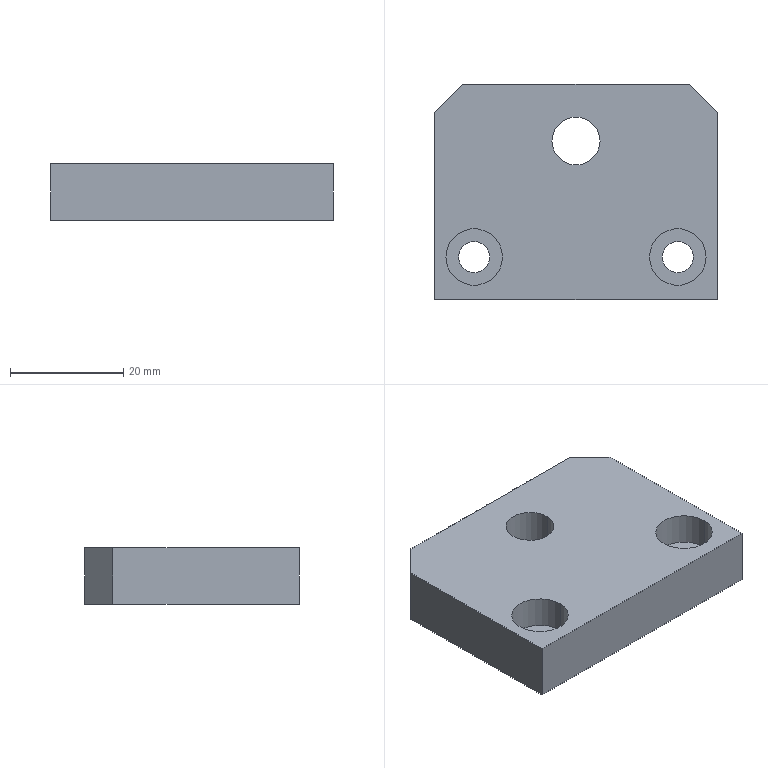Part | STEP file | PN_0016 | 1 solid | 20 faces | box 50 x 38 x 10 mm | volume 17083 mm3 | cylinder 10 | plane 10 | commonest cylinder face diameters 5.5 x4 10 x4 8.5 x2
STEP:
#1=CARTESIAN_POINT('',(0.,0.,0.));
#2=DIRECTION('',(0.,0.,1.));
#3=DIRECTION('',(1.,0.,0.));
#4=AXIS2_PLACEMENT_3D('',#1,#2,#3);
#5=CARTESIAN_POINT('',(-13.,-11.5,-5.7));
#6=VERTEX_POINT('',#5);
#7=CARTESIAN_POINT('',(-13.,-11.5,0.));
#8=VERTEX_POINT('',#7);
#9=CARTESIAN_POINT('',(-13.,-11.5,0.));
#10=DIRECTION('',(0.,0.,1.));
#11=VECTOR('',#10,1.);
#12=LINE('',#9,#11);
#13=CARTESIAN_POINT('',(-18.,-11.5,0.));
#14=DIRECTION('',(0.,0.,1.));
#15=DIRECTION('',(1.,0.,0.));
#16=AXIS2_PLACEMENT_3D('',#13,#14,#15);
#17=CYLINDRICAL_SURFACE('',#16,5.);
#18=CARTESIAN_POINT('',(6.283,0.));
#19=DIRECTION('',(0.,1.));
#20=VECTOR('',#19,1.);
#21=LINE('',#18,#20);
#22=(GEOMETRIC_REPRESENTATION_CONTEXT(2)PARAMETRIC_REPRESENTATION_CONTEXT()REPRESENTATION_CONTEXT('',''));
#23=DEFINITIONAL_REPRESENTATION('',(#21),#22);
#24=PCURVE('',#17,#23);
#25=CARTESIAN_POINT('',(-18.,-11.5,0.));
#26=DIRECTION('',(0.,0.,1.));
#27=DIRECTION('',(1.,0.,0.));
#28=AXIS2_PLACEMENT_3D('',#25,#26,#27);
#29=CYLINDRICAL_SURFACE('',#28,5.);
#30=CARTESIAN_POINT('',(0.,0.));
#31=DIRECTION('',(0.,1.));
#32=VECTOR('',#31,1.);
#33=LINE('',#30,#32);
#34=(GEOMETRIC_REPRESENTATION_CONTEXT(2)PARAMETRIC_REPRESENTATION_CONTEXT()REPRESENTATION_CONTEXT('',''));
#35=DEFINITIONAL_REPRESENTATION('',(#33),#34);
#36=PCURVE('',#29,#35);
#37=SURFACE_CURVE('',#12,(#24,#36),.PCURVE_S1.);
#38=EDGE_CURVE('',#6,#8,#37,.T.);
#39=ORIENTED_EDGE('',*,*,#38,.T.);
#40=CARTESIAN_POINT('',(-23.,-11.5,0.));
#41=VERTEX_POINT('',#40);
#42=CARTESIAN_POINT('',(-18.,-11.5,0.));
#43=DIRECTION('',(0.,0.,1.));
#44=DIRECTION('',(1.,0.,0.));
#45=AXIS2_PLACEMENT_3D('',#42,#43,#44);
#46=CIRCLE('',#45,5.);
#47=CARTESIAN_POINT('',(0.,0.));
#48=DIRECTION('',(1.,0.));
#49=VECTOR('',#48,1.);
#50=LINE('',#47,#49);
#51=(GEOMETRIC_REPRESENTATION_CONTEXT(2)PARAMETRIC_REPRESENTATION_CONTEXT()REPRESENTATION_CONTEXT('',''));
#52=DEFINITIONAL_REPRESENTATION('',(#50),#51);
#53=PCURVE('',#17,#52);
#54=CARTESIAN_POINT('',(0.,0.,0.));
#55=DIRECTION('',(0.,0.,1.));
#56=DIRECTION('',(1.,0.,0.));
#57=AXIS2_PLACEMENT_3D('',#54,#55,#56);
#58=PLANE('',#57);
#59=CARTESIAN_POINT('',(-18.,-11.5));
#60=DIRECTION('',(1.,0.));
#61=AXIS2_PLACEMENT_2D('',#59,#60);
#62=CIRCLE('',#61,5.);
#63=(GEOMETRIC_REPRESENTATION_CONTEXT(2)PARAMETRIC_REPRESENTATION_CONTEXT()REPRESENTATION_CONTEXT('',''));
#64=DEFINITIONAL_REPRESENTATION('',(#62),#63);
#65=PCURVE('',#58,#64);
#66=SURFACE_CURVE('',#46,(#53,#65),.PCURVE_S1.);
#67=EDGE_CURVE('',#41,#8,#66,.T.);
#68=ORIENTED_EDGE('',*,*,#67,.F.);
#69=CARTESIAN_POINT('',(-23.,-11.5,-5.7));
#70=VERTEX_POINT('',#69);
#71=CARTESIAN_POINT('',(-23.,-11.5,0.));
#72=DIRECTION('',(0.,0.,1.));
#73=VECTOR('',#72,1.);
#74=LINE('',#71,#73);
#75=CARTESIAN_POINT('',(3.142,0.));
#76=DIRECTION('',(0.,1.));
#77=VECTOR('',#76,1.);
#78=LINE('',#75,#77);
#79=(GEOMETRIC_REPRESENTATION_CONTEXT(2)PARAMETRIC_REPRESENTATION_CONTEXT()REPRESENTATION_CONTEXT('',''));
#80=DEFINITIONAL_REPRESENTATION('',(#78),#79);
#81=PCURVE('',#17,#80);
#82=CARTESIAN_POINT('',(3.142,0.));
#83=DIRECTION('',(0.,1.));
#84=VECTOR('',#83,1.);
#85=LINE('',#82,#84);
#86=(GEOMETRIC_REPRESENTATION_CONTEXT(2)PARAMETRIC_REPRESENTATION_CONTEXT()REPRESENTATION_CONTEXT('',''));
#87=DEFINITIONAL_REPRESENTATION('',(#85),#86);
#88=PCURVE('',#29,#87);
#89=SURFACE_CURVE('',#74,(#81,#88),.PCURVE_S1.);
#90=EDGE_CURVE('',#70,#41,#89,.T.);
#91=ORIENTED_EDGE('',*,*,#90,.F.);
#92=CARTESIAN_POINT('',(-18.,-11.5,-5.7));
#93=DIRECTION('',(0.,0.,1.));
#94=DIRECTION('',(1.,0.,0.));
#95=AXIS2_PLACEMENT_3D('',#92,#93,#94);
#96=CIRCLE('',#95,5.);
#97=CARTESIAN_POINT('',(0.,-5.7));
#98=DIRECTION('',(1.,0.));
#99=VECTOR('',#98,1.);
#100=LINE('',#97,#99);
#101=(GEOMETRIC_REPRESENTATION_CONTEXT(2)PARAMETRIC_REPRESENTATION_CONTEXT()REPRESENTATION_CONTEXT('',''));
#102=DEFINITIONAL_REPRESENTATION('',(#100),#101);
#103=PCURVE('',#17,#102);
#104=CARTESIAN_POINT('',(-15.25,-11.5,-5.7));
#105=DIRECTION('',(0.,0.,-1.));
#106=DIRECTION('',(-1.,0.,0.));
#107=AXIS2_PLACEMENT_3D('',#104,#105,#106);
#108=PLANE('',#107);
#109=CARTESIAN_POINT('',(-2.25,0.));
#110=CARTESIAN_POINT('',(-2.25,8.66));
#111=CARTESIAN_POINT('',(5.25,4.33));
#112=CARTESIAN_POINT('',(12.75,0.));
#113=CARTESIAN_POINT('',(5.25,-4.33));
#114=CARTESIAN_POINT('',(-2.25,-8.66));
#115=CARTESIAN_POINT('',(-2.25,0.));
#116=(BOUNDED_CURVE()B_SPLINE_CURVE(2,(#109,#110,#111,#112,#113,#114,#115),.UNSPECIFIED.,.T.,.F.)B_SPLINE_CURVE_WITH_KNOTS((1,2,2,2,2,1),(-2.094,0.,2.094,4.189,6.283,8.378),.UNSPECIFIED.)CURVE()GEOMETRIC_REPRESENTATION_ITEM()RATIONAL_B_SPLINE_CURVE((1.,0.5,1.,0.5,1.,0.5,1.))REPRESENTATION_ITEM(''));
#117=(GEOMETRIC_REPRESENTATION_CONTEXT(2)PARAMETRIC_REPRESENTATION_CONTEXT()REPRESENTATION_CONTEXT('',''));
#118=DEFINITIONAL_REPRESENTATION('',(#116),#117);
#119=PCURVE('',#108,#118);
#120=SURFACE_CURVE('',#96,(#103,#119),.PCURVE_S1.);
#121=EDGE_CURVE('',#70,#6,#120,.T.);
#122=ORIENTED_EDGE('',*,*,#121,.T.);
#123=EDGE_LOOP('',(#39,#68,#91,#122));
#124=FACE_BOUND('',#123,.F.);
#125=ADVANCED_FACE('',(#124),#17,.F.);
#126=CARTESIAN_POINT('',(-15.25,-11.5,-10.));
#127=VERTEX_POINT('',#126);
#128=CARTESIAN_POINT('',(-15.25,-11.5,-5.7));
#129=VERTEX_POINT('',#128);
#130=CARTESIAN_POINT('',(-15.25,-11.5,0.));
#131=DIRECTION('',(0.,0.,1.));
#132=VECTOR('',#131,1.);
#133=LINE('',#130,#132);
#134=CARTESIAN_POINT('',(-18.,-11.5,0.));
#135=DIRECTION('',(0.,0.,1.));
#136=DIRECTION('',(1.,0.,0.));
#137=AXIS2_PLACEMENT_3D('',#134,#135,#136);
#138=CYLINDRICAL_SURFACE('',#137,2.75);
#139=CARTESIAN_POINT('',(6.283,0.));
#140=DIRECTION('',(0.,1.));
#141=VECTOR('',#140,1.);
#142=LINE('',#139,#141);
#143=(GEOMETRIC_REPRESENTATION_CONTEXT(2)PARAMETRIC_REPRESENTATION_CONTEXT()REPRESENTATION_CONTEXT('',''));
#144=DEFINITIONAL_REPRESENTATION('',(#142),#143);
#145=PCURVE('',#138,#144);
#146=CARTESIAN_POINT('',(-18.,-11.5,0.));
#147=DIRECTION('',(0.,0.,1.));
#148=DIRECTION('',(1.,0.,0.));
#149=AXIS2_PLACEMENT_3D('',#146,#147,#148);
#150=CYLINDRICAL_SURFACE('',#149,2.75);
#151=CARTESIAN_POINT('',(0.,0.));
#152=DIRECTION('',(0.,1.));
#153=VECTOR('',#152,1.);
#154=LINE('',#151,#153);
#155=(GEOMETRIC_REPRESENTATION_CONTEXT(2)PARAMETRIC_REPRESENTATION_CONTEXT()REPRESENTATION_CONTEXT('',''));
#156=DEFINITIONAL_REPRESENTATION('',(#154),#155);
#157=PCURVE('',#150,#156);
#158=SURFACE_CURVE('',#133,(#145,#157),.PCURVE_S1.);
#159=EDGE_CURVE('',#127,#129,#158,.T.);
#160=ORIENTED_EDGE('',*,*,#159,.T.);
#161=CARTESIAN_POINT('',(-20.75,-11.5,-5.7));
#162=VERTEX_POINT('',#161);
#163=CARTESIAN_POINT('',(-18.,-11.5,-5.7));
#164=DIRECTION('',(0.,0.,1.));
#165=DIRECTION('',(1.,0.,0.));
#166=AXIS2_PLACEMENT_3D('',#163,#164,#165);
#167=CIRCLE('',#166,2.75);
#168=CARTESIAN_POINT('',(0.,-5.7));
#169=DIRECTION('',(1.,0.));
#170=VECTOR('',#169,1.);
#171=LINE('',#168,#170);
#172=(GEOMETRIC_REPRESENTATION_CONTEXT(2)PARAMETRIC_REPRESENTATION_CONTEXT()REPRESENTATION_CONTEXT('',''));
#173=DEFINITIONAL_REPRESENTATION('',(#171),#172);
#174=PCURVE('',#138,#173);
#175=CARTESIAN_POINT('',(0.,0.));
#176=CARTESIAN_POINT('',(0.,4.763));
#177=CARTESIAN_POINT('',(4.125,2.382));
#178=CARTESIAN_POINT('',(8.25,0.));
#179=CARTESIAN_POINT('',(4.125,-2.382));
#180=CARTESIAN_POINT('',(0.,-4.763));
#181=CARTESIAN_POINT('',(0.,0.));
#182=(BOUNDED_CURVE()B_SPLINE_CURVE(2,(#175,#176,#177,#178,#179,#180,#181),.UNSPECIFIED.,.T.,.F.)B_SPLINE_CURVE_WITH_KNOTS((1,2,2,2,2,1),(-2.094,0.,2.094,4.189,6.283,8.378),.UNSPECIFIED.)CURVE()GEOMETRIC_REPRESENTATION_ITEM()RATIONAL_B_SPLINE_CURVE((1.,0.5,1.,0.5,1.,0.5,1.))REPRESENTATION_ITEM(''));
#183=(GEOMETRIC_REPRESENTATION_CONTEXT(2)PARAMETRIC_REPRESENTATION_CONTEXT()REPRESENTATION_CONTEXT('',''));
#184=DEFINITIONAL_REPRESENTATION('',(#182),#183);
#185=PCURVE('',#108,#184);
#186=SURFACE_CURVE('',#167,(#174,#185),.PCURVE_S1.);
#187=EDGE_CURVE('',#162,#129,#186,.T.);
#188=ORIENTED_EDGE('',*,*,#187,.F.);
#189=CARTESIAN_POINT('',(-20.75,-11.5,-10.));
#190=VERTEX_POINT('',#189);
#191=CARTESIAN_POINT('',(-20.75,-11.5,0.));
#192=DIRECTION('',(0.,0.,1.));
#193=VECTOR('',#192,1.);
#194=LINE('',#191,#193);
#195=CARTESIAN_POINT('',(3.142,0.));
#196=DIRECTION('',(0.,1.));
#197=VECTOR('',#196,1.);
#198=LINE('',#195,#197);
#199=(GEOMETRIC_REPRESENTATION_CONTEXT(2)PARAMETRIC_REPRESENTATION_CONTEXT()REPRESENTATION_CONTEXT('',''));
#200=DEFINITIONAL_REPRESENTATION('',(#198),#199);
#201=PCURVE('',#138,#200);
#202=CARTESIAN_POINT('',(3.142,0.));
#203=DIRECTION('',(0.,1.));
#204=VECTOR('',#203,1.);
#205=LINE('',#202,#204);
#206=(GEOMETRIC_REPRESENTATION_CONTEXT(2)PARAMETRIC_REPRESENTATION_CONTEXT()REPRESENTATION_CONTEXT('',''));
#207=DEFINITIONAL_REPRESENTATION('',(#205),#206);
#208=PCURVE('',#150,#207);
#209=SURFACE_CURVE('',#194,(#201,#208),.PCURVE_S1.);
#210=EDGE_CURVE('',#190,#162,#209,.T.);
#211=ORIENTED_EDGE('',*,*,#210,.F.);
#212=CARTESIAN_POINT('',(-18.,-11.5,-10.));
#213=DIRECTION('',(0.,0.,1.));
#214=DIRECTION('',(1.,0.,0.));
#215=AXIS2_PLACEMENT_3D('',#212,#213,#214);
#216=CIRCLE('',#215,2.75);
#217=CARTESIAN_POINT('',(0.,-10.));
#218=DIRECTION('',(1.,0.));
#219=VECTOR('',#218,1.);
#220=LINE('',#217,#219);
#221=(GEOMETRIC_REPRESENTATION_CONTEXT(2)PARAMETRIC_REPRESENTATION_CONTEXT()REPRESENTATION_CONTEXT('',''));
#222=DEFINITIONAL_REPRESENTATION('',(#220),#221);
#223=PCURVE('',#138,#222);
#224=CARTESIAN_POINT('',(0.,0.,-10.));
#225=DIRECTION('',(0.,0.,1.));
#226=DIRECTION('',(1.,0.,0.));
#227=AXIS2_PLACEMENT_3D('',#224,#225,#226);
#228=PLANE('',#227);
#229=CARTESIAN_POINT('',(-18.,-11.5));
#230=DIRECTION('',(1.,0.));
#231=AXIS2_PLACEMENT_2D('',#229,#230);
#232=CIRCLE('',#231,2.75);
#233=(GEOMETRIC_REPRESENTATION_CONTEXT(2)PARAMETRIC_REPRESENTATION_CONTEXT()REPRESENTATION_CONTEXT('',''));
#234=DEFINITIONAL_REPRESENTATION('',(#232),#233);
#235=PCURVE('',#228,#234);
#236=SURFACE_CURVE('',#216,(#223,#235),.PCURVE_S1.);
#237=EDGE_CURVE('',#190,#127,#236,.T.);
#238=ORIENTED_EDGE('',*,*,#237,.T.);
#239=EDGE_LOOP('',(#160,#188,#211,#238));
#240=FACE_BOUND('',#239,.F.);
#241=ADVANCED_FACE('',(#240),#138,.F.);
#242=CARTESIAN_POINT('',(23.,-11.5,-5.7));
#243=VERTEX_POINT('',#242);
#244=CARTESIAN_POINT('',(23.,-11.5,0.));
#245=VERTEX_POINT('',#244);
#246=CARTESIAN_POINT('',(23.,-11.5,0.));
#247=DIRECTION('',(0.,0.,1.));
#248=VECTOR('',#247,1.);
#249=LINE('',#246,#248);
#250=CARTESIAN_POINT('',(18.,-11.5,0.));
#251=DIRECTION('',(0.,0.,1.));
#252=DIRECTION('',(1.,0.,0.));
#253=AXIS2_PLACEMENT_3D('',#250,#251,#252);
#254=CYLINDRICAL_SURFACE('',#253,5.);
#255=CARTESIAN_POINT('',(6.283,0.));
#256=DIRECTION('',(0.,1.));
#257=VECTOR('',#256,1.);
#258=LINE('',#255,#257);
#259=(GEOMETRIC_REPRESENTATION_CONTEXT(2)PARAMETRIC_REPRESENTATION_CONTEXT()REPRESENTATION_CONTEXT('',''));
#260=DEFINITIONAL_REPRESENTATION('',(#258),#259);
#261=PCURVE('',#254,#260);
#262=CARTESIAN_POINT('',(18.,-11.5,0.));
#263=DIRECTION('',(0.,0.,1.));
#264=DIRECTION('',(1.,0.,0.));
#265=AXIS2_PLACEMENT_3D('',#262,#263,#264);
#266=CYLINDRICAL_SURFACE('',#265,5.);
#267=CARTESIAN_POINT('',(0.,0.));
#268=DIRECTION('',(0.,1.));
#269=VECTOR('',#268,1.);
#270=LINE('',#267,#269);
#271=(GEOMETRIC_REPRESENTATION_CONTEXT(2)PARAMETRIC_REPRESENTATION_CONTEXT()REPRESENTATION_CONTEXT('',''));
#272=DEFINITIONAL_REPRESENTATION('',(#270),#271);
#273=PCURVE('',#266,#272);
#274=SURFACE_CURVE('',#249,(#261,#273),.PCURVE_S1.);
#275=EDGE_CURVE('',#243,#245,#274,.T.);
#276=ORIENTED_EDGE('',*,*,#275,.T.);
#277=CARTESIAN_POINT('',(13.,-11.5,0.));
#278=VERTEX_POINT('',#277);
#279=CARTESIAN_POINT('',(18.,-11.5,0.));
#280=DIRECTION('',(0.,0.,1.));
#281=DIRECTION('',(1.,0.,0.));
#282=AXIS2_PLACEMENT_3D('',#279,#280,#281);
#283=CIRCLE('',#282,5.);
#284=CARTESIAN_POINT('',(0.,0.));
#285=DIRECTION('',(1.,0.));
#286=VECTOR('',#285,1.);
#287=LINE('',#284,#286);
#288=(GEOMETRIC_REPRESENTATION_CONTEXT(2)PARAMETRIC_REPRESENTATION_CONTEXT()REPRESENTATION_CONTEXT('',''));
#289=DEFINITIONAL_REPRESENTATION('',(#287),#288);
#290=PCURVE('',#254,#289);
#291=CARTESIAN_POINT('',(18.,-11.5));
#292=DIRECTION('',(1.,0.));
#293=AXIS2_PLACEMENT_2D('',#291,#292);
#294=CIRCLE('',#293,5.);
#295=(GEOMETRIC_REPRESENTATION_CONTEXT(2)PARAMETRIC_REPRESENTATION_CONTEXT()REPRESENTATION_CONTEXT('',''));
#296=DEFINITIONAL_REPRESENTATION('',(#294),#295);
#297=PCURVE('',#58,#296);
#298=SURFACE_CURVE('',#283,(#290,#297),.PCURVE_S1.);
#299=EDGE_CURVE('',#278,#245,#298,.T.);
#300=ORIENTED_EDGE('',*,*,#299,.F.);
#301=CARTESIAN_POINT('',(13.,-11.5,-5.7));
#302=VERTEX_POINT('',#301);
#303=CARTESIAN_POINT('',(13.,-11.5,0.));
#304=DIRECTION('',(0.,0.,1.));
#305=VECTOR('',#304,1.);
#306=LINE('',#303,#305);
#307=CARTESIAN_POINT('',(3.142,0.));
#308=DIRECTION('',(0.,1.));
#309=VECTOR('',#308,1.);
#310=LINE('',#307,#309);
#311=(GEOMETRIC_REPRESENTATION_CONTEXT(2)PARAMETRIC_REPRESENTATION_CONTEXT()REPRESENTATION_CONTEXT('',''));
#312=DEFINITIONAL_REPRESENTATION('',(#310),#311);
#313=PCURVE('',#254,#312);
#314=CARTESIAN_POINT('',(3.142,0.));
#315=DIRECTION('',(0.,1.));
#316=VECTOR('',#315,1.);
#317=LINE('',#314,#316);
#318=(GEOMETRIC_REPRESENTATION_CONTEXT(2)PARAMETRIC_REPRESENTATION_CONTEXT()REPRESENTATION_CONTEXT('',''));
#319=DEFINITIONAL_REPRESENTATION('',(#317),#318);
#320=PCURVE('',#266,#319);
#321=SURFACE_CURVE('',#306,(#313,#320),.PCURVE_S1.);
#322=EDGE_CURVE('',#302,#278,#321,.T.);
#323=ORIENTED_EDGE('',*,*,#322,.F.);
#324=CARTESIAN_POINT('',(18.,-11.5,-5.7));
#325=DIRECTION('',(0.,0.,1.));
#326=DIRECTION('',(1.,0.,0.));
#327=AXIS2_PLACEMENT_3D('',#324,#325,#326);
#328=CIRCLE('',#327,5.);
#329=CARTESIAN_POINT('',(0.,-5.7));
#330=DIRECTION('',(1.,0.));
#331=VECTOR('',#330,1.);
#332=LINE('',#329,#331);
#333=(GEOMETRIC_REPRESENTATION_CONTEXT(2)PARAMETRIC_REPRESENTATION_CONTEXT()REPRESENTATION_CONTEXT('',''));
#334=DEFINITIONAL_REPRESENTATION('',(#332),#333);
#335=PCURVE('',#254,#334);
#336=CARTESIAN_POINT('',(20.75,-11.5,-5.7));
#337=DIRECTION('',(0.,0.,-1.));
#338=DIRECTION('',(-1.,0.,0.));
#339=AXIS2_PLACEMENT_3D('',#336,#337,#338);
#340=PLANE('',#339);
#341=CARTESIAN_POINT('',(-2.25,0.));
#342=CARTESIAN_POINT('',(-2.25,8.66));
#343=CARTESIAN_POINT('',(5.25,4.33));
#344=CARTESIAN_POINT('',(12.75,0.));
#345=CARTESIAN_POINT('',(5.25,-4.33));
#346=CARTESIAN_POINT('',(-2.25,-8.66));
#347=CARTESIAN_POINT('',(-2.25,0.));
#348=(BOUNDED_CURVE()B_SPLINE_CURVE(2,(#341,#342,#343,#344,#345,#346,#347),.UNSPECIFIED.,.T.,.F.)B_SPLINE_CURVE_WITH_KNOTS((1,2,2,2,2,1),(-2.094,0.,2.094,4.189,6.283,8.378),.UNSPECIFIED.)CURVE()GEOMETRIC_REPRESENTATION_ITEM()RATIONAL_B_SPLINE_CURVE((1.,0.5,1.,0.5,1.,0.5,1.))REPRESENTATION_ITEM(''));
#349=(GEOMETRIC_REPRESENTATION_CONTEXT(2)PARAMETRIC_REPRESENTATION_CONTEXT()REPRESENTATION_CONTEXT('',''));
#350=DEFINITIONAL_REPRESENTATION('',(#348),#349);
#351=PCURVE('',#340,#350);
#352=SURFACE_CURVE('',#328,(#335,#351),.PCURVE_S1.);
#353=EDGE_CURVE('',#302,#243,#352,.T.);
#354=ORIENTED_EDGE('',*,*,#353,.T.);
#355=EDGE_LOOP('',(#276,#300,#323,#354));
#356=FACE_BOUND('',#355,.F.);
#357=ADVANCED_FACE('',(#356),#254,.F.);
#358=CARTESIAN_POINT('',(20.75,-11.5,-10.));
#359=VERTEX_POINT('',#358);
#360=CARTESIAN_POINT('',(20.75,-11.5,-5.7));
#361=VERTEX_POINT('',#360);
#362=CARTESIAN_POINT('',(20.75,-11.5,0.));
#363=DIRECTION('',(0.,0.,1.));
#364=VECTOR('',#363,1.);
#365=LINE('',#362,#364);
#366=CARTESIAN_POINT('',(18.,-11.5,0.));
#367=DIRECTION('',(0.,0.,1.));
#368=DIRECTION('',(1.,0.,0.));
#369=AXIS2_PLACEMENT_3D('',#366,#367,#368);
#370=CYLINDRICAL_SURFACE('',#369,2.75);
#371=CARTESIAN_POINT('',(6.283,0.));
#372=DIRECTION('',(0.,1.));
#373=VECTOR('',#372,1.);
#374=LINE('',#371,#373);
#375=(GEOMETRIC_REPRESENTATION_CONTEXT(2)PARAMETRIC_REPRESENTATION_CONTEXT()REPRESENTATION_CONTEXT('',''));
#376=DEFINITIONAL_REPRESENTATION('',(#374),#375);
#377=PCURVE('',#370,#376);
#378=CARTESIAN_POINT('',(18.,-11.5,0.));
#379=DIRECTION('',(0.,0.,1.));
#380=DIRECTION('',(1.,0.,0.));
#381=AXIS2_PLACEMENT_3D('',#378,#379,#380);
#382=CYLINDRICAL_SURFACE('',#381,2.75);
#383=CARTESIAN_POINT('',(0.,0.));
#384=DIRECTION('',(0.,1.));
#385=VECTOR('',#384,1.);
#386=LINE('',#383,#385);
#387=(GEOMETRIC_REPRESENTATION_CONTEXT(2)PARAMETRIC_REPRESENTATION_CONTEXT()REPRESENTATION_CONTEXT('',''));
#388=DEFINITIONAL_REPRESENTATION('',(#386),#387);
#389=PCURVE('',#382,#388);
#390=SURFACE_CURVE('',#365,(#377,#389),.PCURVE_S1.);
#391=EDGE_CURVE('',#359,#361,#390,.T.);
#392=ORIENTED_EDGE('',*,*,#391,.T.);
#393=CARTESIAN_POINT('',(15.25,-11.5,-5.7));
#394=VERTEX_POINT('',#393);
#395=CARTESIAN_POINT('',(18.,-11.5,-5.7));
#396=DIRECTION('',(0.,0.,1.));
#397=DIRECTION('',(1.,0.,0.));
#398=AXIS2_PLACEMENT_3D('',#395,#396,#397);
#399=CIRCLE('',#398,2.75);
#400=CARTESIAN_POINT('',(0.,-5.7));
#401=DIRECTION('',(1.,0.));
#402=VECTOR('',#401,1.);
#403=LINE('',#400,#402);
#404=(GEOMETRIC_REPRESENTATION_CONTEXT(2)PARAMETRIC_REPRESENTATION_CONTEXT()REPRESENTATION_CONTEXT('',''));
#405=DEFINITIONAL_REPRESENTATION('',(#403),#404);
#406=PCURVE('',#370,#405);
#407=CARTESIAN_POINT('',(0.,0.));
#408=CARTESIAN_POINT('',(0.,4.763));
#409=CARTESIAN_POINT('',(4.125,2.382));
#410=CARTESIAN_POINT('',(8.25,0.));
#411=CARTESIAN_POINT('',(4.125,-2.382));
#412=CARTESIAN_POINT('',(0.,-4.763));
#413=CARTESIAN_POINT('',(0.,0.));
#414=(BOUNDED_CURVE()B_SPLINE_CURVE(2,(#407,#408,#409,#410,#411,#412,#413),.UNSPECIFIED.,.T.,.F.)B_SPLINE_CURVE_WITH_KNOTS((1,2,2,2,2,1),(-2.094,0.,2.094,4.189,6.283,8.378),.UNSPECIFIED.)CURVE()GEOMETRIC_REPRESENTATION_ITEM()RATIONAL_B_SPLINE_CURVE((1.,0.5,1.,0.5,1.,0.5,1.))REPRESENTATION_ITEM(''));
#415=(GEOMETRIC_REPRESENTATION_CONTEXT(2)PARAMETRIC_REPRESENTATION_CONTEXT()REPRESENTATION_CONTEXT('',''));
#416=DEFINITIONAL_REPRESENTATION('',(#414),#415);
#417=PCURVE('',#340,#416);
#418=SURFACE_CURVE('',#399,(#406,#417),.PCURVE_S1.);
#419=EDGE_CURVE('',#394,#361,#418,.T.);
#420=ORIENTED_EDGE('',*,*,#419,.F.);
#421=CARTESIAN_POINT('',(15.25,-11.5,-10.));
#422=VERTEX_POINT('',#421);
#423=CARTESIAN_POINT('',(15.25,-11.5,0.));
#424=DIRECTION('',(0.,0.,1.));
#425=VECTOR('',#424,1.);
#426=LINE('',#423,#425);
#427=CARTESIAN_POINT('',(3.142,0.));
#428=DIRECTION('',(0.,1.));
#429=VECTOR('',#428,1.);
#430=LINE('',#427,#429);
#431=(GEOMETRIC_REPRESENTATION_CONTEXT(2)PARAMETRIC_REPRESENTATION_CONTEXT()REPRESENTATION_CONTEXT('',''));
#432=DEFINITIONAL_REPRESENTATION('',(#430),#431);
#433=PCURVE('',#370,#432);
#434=CARTESIAN_POINT('',(3.142,0.));
#435=DIRECTION('',(0.,1.));
#436=VECTOR('',#435,1.);
#437=LINE('',#434,#436);
#438=(GEOMETRIC_REPRESENTATION_CONTEXT(2)PARAMETRIC_REPRESENTATION_CONTEXT()REPRESENTATION_CONTEXT('',''));
#439=DEFINITIONAL_REPRESENTATION('',(#437),#438);
#440=PCURVE('',#382,#439);
#441=SURFACE_CURVE('',#426,(#433,#440),.PCURVE_S1.);
#442=EDGE_CURVE('',#422,#394,#441,.T.);
#443=ORIENTED_EDGE('',*,*,#442,.F.);
#444=CARTESIAN_POINT('',(18.,-11.5,-10.));
#445=DIRECTION('',(0.,0.,1.));
#446=DIRECTION('',(1.,0.,0.));
#447=AXIS2_PLACEMENT_3D('',#444,#445,#446);
#448=CIRCLE('',#447,2.75);
#449=CARTESIAN_POINT('',(0.,-10.));
#450=DIRECTION('',(1.,0.));
#451=VECTOR('',#450,1.);
#452=LINE('',#449,#451);
#453=(GEOMETRIC_REPRESENTATION_CONTEXT(2)PARAMETRIC_REPRESENTATION_CONTEXT()REPRESENTATION_CONTEXT('',''));
#454=DEFINITIONAL_REPRESENTATION('',(#452),#453);
#455=PCURVE('',#370,#454);
#456=CARTESIAN_POINT('',(18.,-11.5));
#457=DIRECTION('',(1.,0.));
#458=AXIS2_PLACEMENT_2D('',#456,#457);
#459=CIRCLE('',#458,2.75);
#460=(GEOMETRIC_REPRESENTATION_CONTEXT(2)PARAMETRIC_REPRESENTATION_CONTEXT()REPRESENTATION_CONTEXT('',''));
#461=DEFINITIONAL_REPRESENTATION('',(#459),#460);
#462=PCURVE('',#228,#461);
#463=SURFACE_CURVE('',#448,(#455,#462),.PCURVE_S1.);
#464=EDGE_CURVE('',#422,#359,#463,.T.);
#465=ORIENTED_EDGE('',*,*,#464,.T.);
#466=EDGE_LOOP('',(#392,#420,#443,#465));
#467=FACE_BOUND('',#466,.F.);
#468=ADVANCED_FACE('',(#467),#370,.F.);
#469=CARTESIAN_POINT('',(4.25,9.,-10.));
#470=VERTEX_POINT('',#469);
#471=CARTESIAN_POINT('',(4.25,9.,0.));
#472=VERTEX_POINT('',#471);
#473=CARTESIAN_POINT('',(4.25,9.,0.));
#474=DIRECTION('',(0.,0.,1.));
#475=VECTOR('',#474,1.);
#476=LINE('',#473,#475);
#477=CARTESIAN_POINT('',(0.,9.,0.));
#478=DIRECTION('',(0.,0.,1.));
#479=DIRECTION('',(1.,0.,0.));
#480=AXIS2_PLACEMENT_3D('',#477,#478,#479);
#481=CYLINDRICAL_SURFACE('',#480,4.25);
#482=CARTESIAN_POINT('',(6.283,0.));
#483=DIRECTION('',(0.,1.));
#484=VECTOR('',#483,1.);
#485=LINE('',#482,#484);
#486=(GEOMETRIC_REPRESENTATION_CONTEXT(2)PARAMETRIC_REPRESENTATION_CONTEXT()REPRESENTATION_CONTEXT('',''));
#487=DEFINITIONAL_REPRESENTATION('',(#485),#486);
#488=PCURVE('',#481,#487);
#489=CARTESIAN_POINT('',(0.,9.,0.));
#490=DIRECTION('',(0.,0.,1.));
#491=DIRECTION('',(1.,0.,0.));
#492=AXIS2_PLACEMENT_3D('',#489,#490,#491);
#493=CYLINDRICAL_SURFACE('',#492,4.25);
#494=CARTESIAN_POINT('',(0.,0.));
#495=DIRECTION('',(0.,1.));
#496=VECTOR('',#495,1.);
#497=LINE('',#494,#496);
#498=(GEOMETRIC_REPRESENTATION_CONTEXT(2)PARAMETRIC_REPRESENTATION_CONTEXT()REPRESENTATION_CONTEXT('',''));
#499=DEFINITIONAL_REPRESENTATION('',(#497),#498);
#500=PCURVE('',#493,#499);
#501=SURFACE_CURVE('',#476,(#488,#500),.PCURVE_S1.);
#502=EDGE_CURVE('',#470,#472,#501,.T.);
#503=ORIENTED_EDGE('',*,*,#502,.T.);
#504=CARTESIAN_POINT('',(-4.25,9.,0.));
#505=VERTEX_POINT('',#504);
#506=CARTESIAN_POINT('',(0.,9.,0.));
#507=DIRECTION('',(0.,0.,1.));
#508=DIRECTION('',(1.,0.,0.));
#509=AXIS2_PLACEMENT_3D('',#506,#507,#508);
#510=CIRCLE('',#509,4.25);
#511=CARTESIAN_POINT('',(0.,0.));
#512=DIRECTION('',(1.,0.));
#513=VECTOR('',#512,1.);
#514=LINE('',#511,#513);
#515=(GEOMETRIC_REPRESENTATION_CONTEXT(2)PARAMETRIC_REPRESENTATION_CONTEXT()REPRESENTATION_CONTEXT('',''));
#516=DEFINITIONAL_REPRESENTATION('',(#514),#515);
#517=PCURVE('',#481,#516);
#518=CARTESIAN_POINT('',(0.,9.));
#519=DIRECTION('',(1.,0.));
#520=AXIS2_PLACEMENT_2D('',#518,#519);
#521=CIRCLE('',#520,4.25);
#522=(GEOMETRIC_REPRESENTATION_CONTEXT(2)PARAMETRIC_REPRESENTATION_CONTEXT()REPRESENTATION_CONTEXT('',''));
#523=DEFINITIONAL_REPRESENTATION('',(#521),#522);
#524=PCURVE('',#58,#523);
#525=SURFACE_CURVE('',#510,(#517,#524),.PCURVE_S1.);
#526=EDGE_CURVE('',#505,#472,#525,.T.);
#527=ORIENTED_EDGE('',*,*,#526,.F.);
#528=CARTESIAN_POINT('',(-4.25,9.,-10.));
#529=VERTEX_POINT('',#528);
#530=CARTESIAN_POINT('',(-4.25,9.,0.));
#531=DIRECTION('',(0.,0.,1.));
#532=VECTOR('',#531,1.);
#533=LINE('',#530,#532);
#534=CARTESIAN_POINT('',(3.142,0.));
#535=DIRECTION('',(0.,1.));
#536=VECTOR('',#535,1.);
#537=LINE('',#534,#536);
#538=(GEOMETRIC_REPRESENTATION_CONTEXT(2)PARAMETRIC_REPRESENTATION_CONTEXT()REPRESENTATION_CONTEXT('',''));
#539=DEFINITIONAL_REPRESENTATION('',(#537),#538);
#540=PCURVE('',#481,#539);
#541=CARTESIAN_POINT('',(3.142,0.));
#542=DIRECTION('',(0.,1.));
#543=VECTOR('',#542,1.);
#544=LINE('',#541,#543);
#545=(GEOMETRIC_REPRESENTATION_CONTEXT(2)PARAMETRIC_REPRESENTATION_CONTEXT()REPRESENTATION_CONTEXT('',''));
#546=DEFINITIONAL_REPRESENTATION('',(#544),#545);
#547=PCURVE('',#493,#546);
#548=SURFACE_CURVE('',#533,(#540,#547),.PCURVE_S1.);
#549=EDGE_CURVE('',#529,#505,#548,.T.);
#550=ORIENTED_EDGE('',*,*,#549,.F.);
#551=CARTESIAN_POINT('',(0.,9.,-10.));
#552=DIRECTION('',(0.,0.,1.));
#553=DIRECTION('',(1.,0.,0.));
#554=AXIS2_PLACEMENT_3D('',#551,#552,#553);
#555=CIRCLE('',#554,4.25);
#556=CARTESIAN_POINT('',(0.,-10.));
#557=DIRECTION('',(1.,0.));
#558=VECTOR('',#557,1.);
#559=LINE('',#556,#558);
#560=(GEOMETRIC_REPRESENTATION_CONTEXT(2)PARAMETRIC_REPRESENTATION_CONTEXT()REPRESENTATION_CONTEXT('',''));
#561=DEFINITIONAL_REPRESENTATION('',(#559),#560);
#562=PCURVE('',#481,#561);
#563=CARTESIAN_POINT('',(0.,9.));
#564=DIRECTION('',(1.,0.));
#565=AXIS2_PLACEMENT_2D('',#563,#564);
#566=CIRCLE('',#565,4.25);
#567=(GEOMETRIC_REPRESENTATION_CONTEXT(2)PARAMETRIC_REPRESENTATION_CONTEXT()REPRESENTATION_CONTEXT('',''));
#568=DEFINITIONAL_REPRESENTATION('',(#566),#567);
#569=PCURVE('',#228,#568);
#570=SURFACE_CURVE('',#555,(#562,#569),.PCURVE_S1.);
#571=EDGE_CURVE('',#529,#470,#570,.T.);
#572=ORIENTED_EDGE('',*,*,#571,.T.);
#573=EDGE_LOOP('',(#503,#527,#550,#572));
#574=FACE_BOUND('',#573,.F.);
#575=ADVANCED_FACE('',(#574),#481,.F.);
#576=CARTESIAN_POINT('',(25.,-19.,-10.));
#577=VERTEX_POINT('',#576);
#578=CARTESIAN_POINT('',(25.,14.,-10.));
#579=VERTEX_POINT('',#578);
#580=CARTESIAN_POINT('',(25.,19.,-10.));
#581=DIRECTION('',(0.,1.,0.));
#582=VECTOR('',#581,1.);
#583=LINE('',#580,#582);
#584=CARTESIAN_POINT('',(25.,19.,-10.));
#585=DIRECTION('',(1.,0.,0.));
#586=DIRECTION('',(0.,1.,0.));
#587=AXIS2_PLACEMENT_3D('',#584,#585,#586);
#588=PLANE('',#587);
#589=CARTESIAN_POINT('',(0.,0.));
#590=DIRECTION('',(1.,0.));
#591=VECTOR('',#590,1.);
#592=LINE('',#589,#591);
#593=(GEOMETRIC_REPRESENTATION_CONTEXT(2)PARAMETRIC_REPRESENTATION_CONTEXT()REPRESENTATION_CONTEXT('',''));
#594=DEFINITIONAL_REPRESENTATION('',(#592),#593);
#595=PCURVE('',#588,#594);
#596=CARTESIAN_POINT('',(25.,19.));
#597=DIRECTION('',(0.,1.));
#598=VECTOR('',#597,1.);
#599=LINE('',#596,#598);
#600=(GEOMETRIC_REPRESENTATION_CONTEXT(2)PARAMETRIC_REPRESENTATION_CONTEXT()REPRESENTATION_CONTEXT('',''));
#601=DEFINITIONAL_REPRESENTATION('',(#599),#600);
#602=PCURVE('',#228,#601);
#603=SURFACE_CURVE('',#583,(#595,#602),.PCURVE_S1.);
#604=EDGE_CURVE('',#577,#579,#603,.T.);
#605=ORIENTED_EDGE('',*,*,#604,.T.);
#606=CARTESIAN_POINT('',(25.,14.,0.));
#607=VERTEX_POINT('',#606);
#608=CARTESIAN_POINT('',(25.,14.,-10.));
#609=DIRECTION('',(0.,0.,1.));
#610=VECTOR('',#609,1.);
#611=LINE('',#608,#610);
#612=CARTESIAN_POINT('',(-5.,0.));
#613=DIRECTION('',(0.,1.));
#614=VECTOR('',#613,1.);
#615=LINE('',#612,#614);
#616=(GEOMETRIC_REPRESENTATION_CONTEXT(2)PARAMETRIC_REPRESENTATION_CONTEXT()REPRESENTATION_CONTEXT('',''));
#617=DEFINITIONAL_REPRESENTATION('',(#615),#616);
#618=PCURVE('',#588,#617);
#619=CARTESIAN_POINT('',(25.,14.,-10.));
#620=DIRECTION('',(-0.7071,-0.7071,0.));
#621=DIRECTION('',(0.,0.,1.));
#622=AXIS2_PLACEMENT_3D('',#619,#620,#621);
#623=PLANE('',#622);
#624=CARTESIAN_POINT('',(0.,0.));
#625=DIRECTION('',(1.,0.));
#626=VECTOR('',#625,1.);
#627=LINE('',#624,#626);
#628=(GEOMETRIC_REPRESENTATION_CONTEXT(2)PARAMETRIC_REPRESENTATION_CONTEXT()REPRESENTATION_CONTEXT('',''));
#629=DEFINITIONAL_REPRESENTATION('',(#627),#628);
#630=PCURVE('',#623,#629);
#631=SURFACE_CURVE('',#611,(#618,#630),.PCURVE_S1.);
#632=EDGE_CURVE('',#579,#607,#631,.T.);
#633=ORIENTED_EDGE('',*,*,#632,.T.);
#634=CARTESIAN_POINT('',(25.,-19.,0.));
#635=VERTEX_POINT('',#634);
#636=CARTESIAN_POINT('',(25.,19.,0.));
#637=DIRECTION('',(0.,1.,0.));
#638=VECTOR('',#637,1.);
#639=LINE('',#636,#638);
#640=CARTESIAN_POINT('',(0.,10.));
#641=DIRECTION('',(1.,0.));
#642=VECTOR('',#641,1.);
#643=LINE('',#640,#642);
#644=(GEOMETRIC_REPRESENTATION_CONTEXT(2)PARAMETRIC_REPRESENTATION_CONTEXT()REPRESENTATION_CONTEXT('',''));
#645=DEFINITIONAL_REPRESENTATION('',(#643),#644);
#646=PCURVE('',#588,#645);
#647=CARTESIAN_POINT('',(25.,19.));
#648=DIRECTION('',(0.,1.));
#649=VECTOR('',#648,1.);
#650=LINE('',#647,#649);
#651=(GEOMETRIC_REPRESENTATION_CONTEXT(2)PARAMETRIC_REPRESENTATION_CONTEXT()REPRESENTATION_CONTEXT('',''));
#652=DEFINITIONAL_REPRESENTATION('',(#650),#651);
#653=PCURVE('',#58,#652);
#654=SURFACE_CURVE('',#639,(#646,#653),.PCURVE_S1.);
#655=EDGE_CURVE('',#635,#607,#654,.T.);
#656=ORIENTED_EDGE('',*,*,#655,.F.);
#657=CARTESIAN_POINT('',(25.,-19.,-10.));
#658=DIRECTION('',(0.,0.,1.));
#659=VECTOR('',#658,1.);
#660=LINE('',#657,#659);
#661=CARTESIAN_POINT('',(-38.,0.));
#662=DIRECTION('',(0.,1.));
#663=VECTOR('',#662,1.);
#664=LINE('',#661,#663);
#665=(GEOMETRIC_REPRESENTATION_CONTEXT(2)PARAMETRIC_REPRESENTATION_CONTEXT()REPRESENTATION_CONTEXT('',''));
#666=DEFINITIONAL_REPRESENTATION('',(#664),#665);
#667=PCURVE('',#588,#666);
#668=CARTESIAN_POINT('',(-25.,-19.,-10.));
#669=DIRECTION('',(0.,-1.,0.));
#670=DIRECTION('',(0.,0.,-1.));
#671=AXIS2_PLACEMENT_3D('',#668,#669,#670);
#672=PLANE('',#671);
#673=CARTESIAN_POINT('',(0.,50.));
#674=DIRECTION('',(-1.,0.));
#675=VECTOR('',#674,1.);
#676=LINE('',#673,#675);
#677=(GEOMETRIC_REPRESENTATION_CONTEXT(2)PARAMETRIC_REPRESENTATION_CONTEXT()REPRESENTATION_CONTEXT('',''));
#678=DEFINITIONAL_REPRESENTATION('',(#676),#677);
#679=PCURVE('',#672,#678);
#680=SURFACE_CURVE('',#660,(#667,#679),.PCURVE_S1.);
#681=EDGE_CURVE('',#577,#635,#680,.T.);
#682=ORIENTED_EDGE('',*,*,#681,.F.);
#683=EDGE_LOOP('',(#605,#633,#656,#682));
#684=FACE_BOUND('',#683,.T.);
#685=ADVANCED_FACE('',(#684),#588,.T.);
#686=CARTESIAN_POINT('',(-25.,-19.,0.));
#687=VERTEX_POINT('',#686);
#688=CARTESIAN_POINT('',(-25.,-19.,0.));
#689=DIRECTION('',(1.,0.,0.));
#690=VECTOR('',#689,1.);
#691=LINE('',#688,#690);
#692=CARTESIAN_POINT('',(-10.,0.));
#693=DIRECTION('',(0.,1.));
#694=VECTOR('',#693,1.);
#695=LINE('',#692,#694);
#696=(GEOMETRIC_REPRESENTATION_CONTEXT(2)PARAMETRIC_REPRESENTATION_CONTEXT()REPRESENTATION_CONTEXT('',''));
#697=DEFINITIONAL_REPRESENTATION('',(#695),#696);
#698=PCURVE('',#672,#697);
#699=CARTESIAN_POINT('',(-25.,-19.));
#700=DIRECTION('',(1.,0.));
#701=VECTOR('',#700,1.);
#702=LINE('',#699,#701);
#703=(GEOMETRIC_REPRESENTATION_CONTEXT(2)PARAMETRIC_REPRESENTATION_CONTEXT()REPRESENTATION_CONTEXT('',''));
#704=DEFINITIONAL_REPRESENTATION('',(#702),#703);
#705=PCURVE('',#58,#704);
#706=SURFACE_CURVE('',#691,(#698,#705),.PCURVE_S1.);
#707=EDGE_CURVE('',#687,#635,#706,.T.);
#708=ORIENTED_EDGE('',*,*,#707,.F.);
#709=CARTESIAN_POINT('',(-25.,-19.,-10.));
#710=VERTEX_POINT('',#709);
#711=CARTESIAN_POINT('',(-25.,-19.,-10.));
#712=DIRECTION('',(0.,0.,1.));
#713=VECTOR('',#712,1.);
#714=LINE('',#711,#713);
#715=CARTESIAN_POINT('',(0.,0.));
#716=DIRECTION('',(-1.,0.));
#717=VECTOR('',#716,1.);
#718=LINE('',#715,#717);
#719=(GEOMETRIC_REPRESENTATION_CONTEXT(2)PARAMETRIC_REPRESENTATION_CONTEXT()REPRESENTATION_CONTEXT('',''));
#720=DEFINITIONAL_REPRESENTATION('',(#718),#719);
#721=PCURVE('',#672,#720);
#722=CARTESIAN_POINT('',(-25.,19.,-10.));
#723=DIRECTION('',(-1.,0.,0.));
#724=DIRECTION('',(0.,-1.,0.));
#725=AXIS2_PLACEMENT_3D('',#722,#723,#724);
#726=PLANE('',#725);
#727=CARTESIAN_POINT('',(38.,0.));
#728=DIRECTION('',(0.,1.));
#729=VECTOR('',#728,1.);
#730=LINE('',#727,#729);
#731=(GEOMETRIC_REPRESENTATION_CONTEXT(2)PARAMETRIC_REPRESENTATION_CONTEXT()REPRESENTATION_CONTEXT('',''));
#732=DEFINITIONAL_REPRESENTATION('',(#730),#731);
#733=PCURVE('',#726,#732);
#734=SURFACE_CURVE('',#714,(#721,#733),.PCURVE_S1.);
#735=EDGE_CURVE('',#710,#687,#734,.T.);
#736=ORIENTED_EDGE('',*,*,#735,.F.);
#737=CARTESIAN_POINT('',(-25.,-19.,-10.));
#738=DIRECTION('',(1.,0.,0.));
#739=VECTOR('',#738,1.);
#740=LINE('',#737,#739);
#741=CARTESIAN_POINT('',(0.,0.));
#742=DIRECTION('',(0.,1.));
#743=VECTOR('',#742,1.);
#744=LINE('',#741,#743);
#745=(GEOMETRIC_REPRESENTATION_CONTEXT(2)PARAMETRIC_REPRESENTATION_CONTEXT()REPRESENTATION_CONTEXT('',''));
#746=DEFINITIONAL_REPRESENTATION('',(#744),#745);
#747=PCURVE('',#672,#746);
#748=CARTESIAN_POINT('',(-25.,-19.));
#749=DIRECTION('',(1.,0.));
#750=VECTOR('',#749,1.);
#751=LINE('',#748,#750);
#752=(GEOMETRIC_REPRESENTATION_CONTEXT(2)PARAMETRIC_REPRESENTATION_CONTEXT()REPRESENTATION_CONTEXT('',''));
#753=DEFINITIONAL_REPRESENTATION('',(#751),#752);
#754=PCURVE('',#228,#753);
#755=SURFACE_CURVE('',#740,(#747,#754),.PCURVE_S1.);
#756=EDGE_CURVE('',#710,#577,#755,.T.);
#757=ORIENTED_EDGE('',*,*,#756,.T.);
#758=ORIENTED_EDGE('',*,*,#681,.T.);
#759=EDGE_LOOP('',(#708,#736,#757,#758));
#760=FACE_BOUND('',#759,.T.);
#761=ADVANCED_FACE('',(#760),#672,.T.);
#762=CARTESIAN_POINT('',(-25.,14.,0.));
#763=VERTEX_POINT('',#762);
#764=CARTESIAN_POINT('',(-25.,19.,0.));
#765=DIRECTION('',(0.,-1.,0.));
#766=VECTOR('',#765,1.);
#767=LINE('',#764,#766);
#768=CARTESIAN_POINT('',(0.,10.));
#769=DIRECTION('',(1.,0.));
#770=VECTOR('',#769,1.);
#771=LINE('',#768,#770);
#772=(GEOMETRIC_REPRESENTATION_CONTEXT(2)PARAMETRIC_REPRESENTATION_CONTEXT()REPRESENTATION_CONTEXT('',''));
#773=DEFINITIONAL_REPRESENTATION('',(#771),#772);
#774=PCURVE('',#726,#773);
#775=CARTESIAN_POINT('',(-25.,19.));
#776=DIRECTION('',(0.,-1.));
#777=VECTOR('',#776,1.);
#778=LINE('',#775,#777);
#779=(GEOMETRIC_REPRESENTATION_CONTEXT(2)PARAMETRIC_REPRESENTATION_CONTEXT()REPRESENTATION_CONTEXT('',''));
#780=DEFINITIONAL_REPRESENTATION('',(#778),#779);
#781=PCURVE('',#58,#780);
#782=SURFACE_CURVE('',#767,(#774,#781),.PCURVE_S1.);
#783=EDGE_CURVE('',#763,#687,#782,.T.);
#784=ORIENTED_EDGE('',*,*,#783,.F.);
#785=CARTESIAN_POINT('',(-25.,14.,-10.));
#786=VERTEX_POINT('',#785);
#787=CARTESIAN_POINT('',(-25.,14.,-10.));
#788=DIRECTION('',(0.,0.,-1.));
#789=VECTOR('',#788,1.);
#790=LINE('',#787,#789);
#791=CARTESIAN_POINT('',(5.,0.));
#792=DIRECTION('',(0.,-1.));
#793=VECTOR('',#792,1.);
#794=LINE('',#791,#793);
#795=(GEOMETRIC_REPRESENTATION_CONTEXT(2)PARAMETRIC_REPRESENTATION_CONTEXT()REPRESENTATION_CONTEXT('',''));
#796=DEFINITIONAL_REPRESENTATION('',(#794),#795);
#797=PCURVE('',#726,#796);
#798=CARTESIAN_POINT('',(-20.,19.,-10.));
#799=DIRECTION('',(0.7071,-0.7071,0.));
#800=DIRECTION('',(0.,0.,1.));
#801=AXIS2_PLACEMENT_3D('',#798,#799,#800);
#802=PLANE('',#801);
#803=CARTESIAN_POINT('',(0.,7.071));
#804=DIRECTION('',(-1.,0.));
#805=VECTOR('',#804,1.);
#806=LINE('',#803,#805);
#807=(GEOMETRIC_REPRESENTATION_CONTEXT(2)PARAMETRIC_REPRESENTATION_CONTEXT()REPRESENTATION_CONTEXT('',''));
#808=DEFINITIONAL_REPRESENTATION('',(#806),#807);
#809=PCURVE('',#802,#808);
#810=SURFACE_CURVE('',#790,(#797,#809),.PCURVE_S1.);
#811=EDGE_CURVE('',#763,#786,#810,.T.);
#812=ORIENTED_EDGE('',*,*,#811,.T.);
#813=CARTESIAN_POINT('',(-25.,19.,-10.));
#814=DIRECTION('',(0.,-1.,0.));
#815=VECTOR('',#814,1.);
#816=LINE('',#813,#815);
#817=CARTESIAN_POINT('',(0.,0.));
#818=DIRECTION('',(1.,0.));
#819=VECTOR('',#818,1.);
#820=LINE('',#817,#819);
#821=(GEOMETRIC_REPRESENTATION_CONTEXT(2)PARAMETRIC_REPRESENTATION_CONTEXT()REPRESENTATION_CONTEXT('',''));
#822=DEFINITIONAL_REPRESENTATION('',(#820),#821);
#823=PCURVE('',#726,#822);
#824=CARTESIAN_POINT('',(-25.,19.));
#825=DIRECTION('',(0.,-1.));
#826=VECTOR('',#825,1.);
#827=LINE('',#824,#826);
#828=(GEOMETRIC_REPRESENTATION_CONTEXT(2)PARAMETRIC_REPRESENTATION_CONTEXT()REPRESENTATION_CONTEXT('',''));
#829=DEFINITIONAL_REPRESENTATION('',(#827),#828);
#830=PCURVE('',#228,#829);
#831=SURFACE_CURVE('',#816,(#823,#830),.PCURVE_S1.);
#832=EDGE_CURVE('',#786,#710,#831,.T.);
#833=ORIENTED_EDGE('',*,*,#832,.T.);
#834=ORIENTED_EDGE('',*,*,#735,.T.);
#835=EDGE_LOOP('',(#784,#812,#833,#834));
#836=FACE_BOUND('',#835,.T.);
#837=ADVANCED_FACE('',(#836),#726,.T.);
#838=CARTESIAN_POINT('',(20.,19.,0.));
#839=VERTEX_POINT('',#838);
#840=CARTESIAN_POINT('',(-20.,19.,0.));
#841=VERTEX_POINT('',#840);
#842=CARTESIAN_POINT('',(-25.,19.,0.));
#843=DIRECTION('',(-1.,0.,0.));
#844=VECTOR('',#843,1.);
#845=LINE('',#842,#844);
#846=CARTESIAN_POINT('',(-25.,19.,-10.));
#847=DIRECTION('',(0.,1.,0.));
#848=DIRECTION('',(0.,0.,1.));
#849=AXIS2_PLACEMENT_3D('',#846,#847,#848);
#850=PLANE('',#849);
#851=CARTESIAN_POINT('',(10.,0.));
#852=DIRECTION('',(0.,-1.));
#853=VECTOR('',#852,1.);
#854=LINE('',#851,#853);
#855=(GEOMETRIC_REPRESENTATION_CONTEXT(2)PARAMETRIC_REPRESENTATION_CONTEXT()REPRESENTATION_CONTEXT('',''));
#856=DEFINITIONAL_REPRESENTATION('',(#854),#855);
#857=PCURVE('',#850,#856);
#858=CARTESIAN_POINT('',(-25.,19.));
#859=DIRECTION('',(-1.,0.));
#860=VECTOR('',#859,1.);
#861=LINE('',#858,#860);
#862=(GEOMETRIC_REPRESENTATION_CONTEXT(2)PARAMETRIC_REPRESENTATION_CONTEXT()REPRESENTATION_CONTEXT('',''));
#863=DEFINITIONAL_REPRESENTATION('',(#861),#862);
#864=PCURVE('',#58,#863);
#865=SURFACE_CURVE('',#845,(#857,#864),.PCURVE_S1.);
#866=EDGE_CURVE('',#839,#841,#865,.T.);
#867=ORIENTED_EDGE('',*,*,#866,.F.);
#868=CARTESIAN_POINT('',(20.,19.,-10.));
#869=VERTEX_POINT('',#868);
#870=CARTESIAN_POINT('',(20.,19.,-10.));
#871=DIRECTION('',(0.,0.,-1.));
#872=VECTOR('',#871,1.);
#873=LINE('',#870,#872);
#874=CARTESIAN_POINT('',(0.,45.));
#875=DIRECTION('',(-1.,0.));
#876=VECTOR('',#875,1.);
#877=LINE('',#874,#876);
#878=(GEOMETRIC_REPRESENTATION_CONTEXT(2)PARAMETRIC_REPRESENTATION_CONTEXT()REPRESENTATION_CONTEXT('',''));
#879=DEFINITIONAL_REPRESENTATION('',(#877),#878);
#880=PCURVE('',#850,#879);
#881=CARTESIAN_POINT('',(0.,7.071));
#882=DIRECTION('',(-1.,0.));
#883=VECTOR('',#882,1.);
#884=LINE('',#881,#883);
#885=(GEOMETRIC_REPRESENTATION_CONTEXT(2)PARAMETRIC_REPRESENTATION_CONTEXT()REPRESENTATION_CONTEXT('',''));
#886=DEFINITIONAL_REPRESENTATION('',(#884),#885);
#887=PCURVE('',#623,#886);
#888=SURFACE_CURVE('',#873,(#880,#887),.PCURVE_S1.);
#889=EDGE_CURVE('',#839,#869,#888,.T.);
#890=ORIENTED_EDGE('',*,*,#889,.T.);
#891=CARTESIAN_POINT('',(-20.,19.,-10.));
#892=VERTEX_POINT('',#891);
#893=CARTESIAN_POINT('',(-25.,19.,-10.));
#894=DIRECTION('',(-1.,0.,0.));
#895=VECTOR('',#894,1.);
#896=LINE('',#893,#895);
#897=CARTESIAN_POINT('',(0.,0.));
#898=DIRECTION('',(0.,-1.));
#899=VECTOR('',#898,1.);
#900=LINE('',#897,#899);
#901=(GEOMETRIC_REPRESENTATION_CONTEXT(2)PARAMETRIC_REPRESENTATION_CONTEXT()REPRESENTATION_CONTEXT('',''));
#902=DEFINITIONAL_REPRESENTATION('',(#900),#901);
#903=PCURVE('',#850,#902);
#904=CARTESIAN_POINT('',(-25.,19.));
#905=DIRECTION('',(-1.,0.));
#906=VECTOR('',#905,1.);
#907=LINE('',#904,#906);
#908=(GEOMETRIC_REPRESENTATION_CONTEXT(2)PARAMETRIC_REPRESENTATION_CONTEXT()REPRESENTATION_CONTEXT('',''));
#909=DEFINITIONAL_REPRESENTATION('',(#907),#908);
#910=PCURVE('',#228,#909);
#911=SURFACE_CURVE('',#896,(#903,#910),.PCURVE_S1.);
#912=EDGE_CURVE('',#869,#892,#911,.T.);
#913=ORIENTED_EDGE('',*,*,#912,.T.);
#914=CARTESIAN_POINT('',(-20.,19.,-10.));
#915=DIRECTION('',(0.,0.,1.));
#916=VECTOR('',#915,1.);
#917=LINE('',#914,#916);
#918=CARTESIAN_POINT('',(0.,5.));
#919=DIRECTION('',(1.,0.));
#920=VECTOR('',#919,1.);
#921=LINE('',#918,#920);
#922=(GEOMETRIC_REPRESENTATION_CONTEXT(2)PARAMETRIC_REPRESENTATION_CONTEXT()REPRESENTATION_CONTEXT('',''));
#923=DEFINITIONAL_REPRESENTATION('',(#921),#922);
#924=PCURVE('',#850,#923);
#925=CARTESIAN_POINT('',(0.,0.));
#926=DIRECTION('',(1.,0.));
#927=VECTOR('',#926,1.);
#928=LINE('',#925,#927);
#929=(GEOMETRIC_REPRESENTATION_CONTEXT(2)PARAMETRIC_REPRESENTATION_CONTEXT()REPRESENTATION_CONTEXT('',''));
#930=DEFINITIONAL_REPRESENTATION('',(#928),#929);
#931=PCURVE('',#802,#930);
#932=SURFACE_CURVE('',#917,(#924,#931),.PCURVE_S1.);
#933=EDGE_CURVE('',#892,#841,#932,.T.);
#934=ORIENTED_EDGE('',*,*,#933,.T.);
#935=EDGE_LOOP('',(#867,#890,#913,#934));
#936=FACE_BOUND('',#935,.T.);
#937=ADVANCED_FACE('',(#936),#850,.T.);
#938=CARTESIAN_POINT('',(-18.,-11.5,-10.));
#939=DIRECTION('',(0.,0.,1.));
#940=DIRECTION('',(1.,0.,0.));
#941=AXIS2_PLACEMENT_3D('',#938,#939,#940);
#942=CIRCLE('',#941,2.75);
#943=CARTESIAN_POINT('',(-18.,-11.5));
#944=DIRECTION('',(1.,0.));
#945=AXIS2_PLACEMENT_2D('',#943,#944);
#946=CIRCLE('',#945,2.75);
#947=(GEOMETRIC_REPRESENTATION_CONTEXT(2)PARAMETRIC_REPRESENTATION_CONTEXT()REPRESENTATION_CONTEXT('',''));
#948=DEFINITIONAL_REPRESENTATION('',(#946),#947);
#949=PCURVE('',#228,#948);
#950=CARTESIAN_POINT('',(0.,-10.));
#951=DIRECTION('',(1.,0.));
#952=VECTOR('',#951,1.);
#953=LINE('',#950,#952);
#954=(GEOMETRIC_REPRESENTATION_CONTEXT(2)PARAMETRIC_REPRESENTATION_CONTEXT()REPRESENTATION_CONTEXT('',''));
#955=DEFINITIONAL_REPRESENTATION('',(#953),#954);
#956=PCURVE('',#150,#955);
#957=SURFACE_CURVE('',#942,(#949,#956),.PCURVE_S1.);
#958=EDGE_CURVE('',#127,#190,#957,.T.);
#959=ORIENTED_EDGE('',*,*,#958,.T.);
#960=ORIENTED_EDGE('',*,*,#237,.T.);
#961=EDGE_LOOP('',(#959,#960));
#962=FACE_BOUND('',#961,.T.);
#963=CARTESIAN_POINT('',(18.,-11.5,-10.));
#964=DIRECTION('',(0.,0.,1.));
#965=DIRECTION('',(1.,0.,0.));
#966=AXIS2_PLACEMENT_3D('',#963,#964,#965);
#967=CIRCLE('',#966,2.75);
#968=CARTESIAN_POINT('',(18.,-11.5));
#969=DIRECTION('',(1.,0.));
#970=AXIS2_PLACEMENT_2D('',#968,#969);
#971=CIRCLE('',#970,2.75);
#972=(GEOMETRIC_REPRESENTATION_CONTEXT(2)PARAMETRIC_REPRESENTATION_CONTEXT()REPRESENTATION_CONTEXT('',''));
#973=DEFINITIONAL_REPRESENTATION('',(#971),#972);
#974=PCURVE('',#228,#973);
#975=CARTESIAN_POINT('',(0.,-10.));
#976=DIRECTION('',(1.,0.));
#977=VECTOR('',#976,1.);
#978=LINE('',#975,#977);
#979=(GEOMETRIC_REPRESENTATION_CONTEXT(2)PARAMETRIC_REPRESENTATION_CONTEXT()REPRESENTATION_CONTEXT('',''));
#980=DEFINITIONAL_REPRESENTATION('',(#978),#979);
#981=PCURVE('',#382,#980);
#982=SURFACE_CURVE('',#967,(#974,#981),.PCURVE_S1.);
#983=EDGE_CURVE('',#359,#422,#982,.T.);
#984=ORIENTED_EDGE('',*,*,#983,.T.);
#985=ORIENTED_EDGE('',*,*,#464,.T.);
#986=EDGE_LOOP('',(#984,#985));
#987=FACE_BOUND('',#986,.T.);
#988=CARTESIAN_POINT('',(0.,9.,-10.));
#989=DIRECTION('',(0.,0.,1.));
#990=DIRECTION('',(1.,0.,0.));
#991=AXIS2_PLACEMENT_3D('',#988,#989,#990);
#992=CIRCLE('',#991,4.25);
#993=CARTESIAN_POINT('',(0.,9.));
#994=DIRECTION('',(1.,0.));
#995=AXIS2_PLACEMENT_2D('',#993,#994);
#996=CIRCLE('',#995,4.25);
#997=(GEOMETRIC_REPRESENTATION_CONTEXT(2)PARAMETRIC_REPRESENTATION_CONTEXT()REPRESENTATION_CONTEXT('',''));
#998=DEFINITIONAL_REPRESENTATION('',(#996),#997);
#999=PCURVE('',#228,#998);
#1000=CARTESIAN_POINT('',(0.,-10.));
#1001=DIRECTION('',(1.,0.));
#1002=VECTOR('',#1001,1.);
#1003=LINE('',#1000,#1002);
#1004=(GEOMETRIC_REPRESENTATION_CONTEXT(2)PARAMETRIC_REPRESENTATION_CONTEXT()REPRESENTATION_CONTEXT('',''));
#1005=DEFINITIONAL_REPRESENTATION('',(#1003),#1004);
#1006=PCURVE('',#493,#1005);
#1007=SURFACE_CURVE('',#992,(#999,#1006),.PCURVE_S1.);
#1008=EDGE_CURVE('',#470,#529,#1007,.T.);
#1009=ORIENTED_EDGE('',*,*,#1008,.T.);
#1010=ORIENTED_EDGE('',*,*,#571,.T.);
#1011=EDGE_LOOP('',(#1009,#1010));
#1012=FACE_BOUND('',#1011,.T.);
#1013=ORIENTED_EDGE('',*,*,#912,.F.);
#1014=CARTESIAN_POINT('',(25.,14.,-10.));
#1015=DIRECTION('',(0.7071,-0.7071,0.));
#1016=VECTOR('',#1015,1.);
#1017=LINE('',#1014,#1016);
#1018=CARTESIAN_POINT('',(25.,14.));
#1019=DIRECTION('',(0.7071,-0.7071));
#1020=VECTOR('',#1019,1.);
#1021=LINE('',#1018,#1020);
#1022=(GEOMETRIC_REPRESENTATION_CONTEXT(2)PARAMETRIC_REPRESENTATION_CONTEXT()REPRESENTATION_CONTEXT('',''));
#1023=DEFINITIONAL_REPRESENTATION('',(#1021),#1022);
#1024=PCURVE('',#228,#1023);
#1025=CARTESIAN_POINT('',(0.,0.));
#1026=DIRECTION('',(0.,-1.));
#1027=VECTOR('',#1026,1.);
#1028=LINE('',#1025,#1027);
#1029=(GEOMETRIC_REPRESENTATION_CONTEXT(2)PARAMETRIC_REPRESENTATION_CONTEXT()REPRESENTATION_CONTEXT('',''));
#1030=DEFINITIONAL_REPRESENTATION('',(#1028),#1029);
#1031=PCURVE('',#623,#1030);
#1032=SURFACE_CURVE('',#1017,(#1024,#1031),.PCURVE_S1.);
#1033=EDGE_CURVE('',#869,#579,#1032,.T.);
#1034=ORIENTED_EDGE('',*,*,#1033,.T.);
#1035=ORIENTED_EDGE('',*,*,#604,.F.);
#1036=ORIENTED_EDGE('',*,*,#756,.F.);
#1037=ORIENTED_EDGE('',*,*,#832,.F.);
#1038=CARTESIAN_POINT('',(-20.,19.,-10.));
#1039=DIRECTION('',(0.7071,0.7071,0.));
#1040=VECTOR('',#1039,1.);
#1041=LINE('',#1038,#1040);
#1042=CARTESIAN_POINT('',(-20.,19.));
#1043=DIRECTION('',(0.7071,0.7071));
#1044=VECTOR('',#1043,1.);
#1045=LINE('',#1042,#1044);
#1046=(GEOMETRIC_REPRESENTATION_CONTEXT(2)PARAMETRIC_REPRESENTATION_CONTEXT()REPRESENTATION_CONTEXT('',''));
#1047=DEFINITIONAL_REPRESENTATION('',(#1045),#1046);
#1048=PCURVE('',#228,#1047);
#1049=CARTESIAN_POINT('',(0.,0.));
#1050=DIRECTION('',(0.,-1.));
#1051=VECTOR('',#1050,1.);
#1052=LINE('',#1049,#1051);
#1053=(GEOMETRIC_REPRESENTATION_CONTEXT(2)PARAMETRIC_REPRESENTATION_CONTEXT()REPRESENTATION_CONTEXT('',''));
#1054=DEFINITIONAL_REPRESENTATION('',(#1052),#1053);
#1055=PCURVE('',#802,#1054);
#1056=SURFACE_CURVE('',#1041,(#1048,#1055),.PCURVE_S1.);
#1057=EDGE_CURVE('',#786,#892,#1056,.T.);
#1058=ORIENTED_EDGE('',*,*,#1057,.T.);
#1059=EDGE_LOOP('',(#1013,#1034,#1035,#1036,#1037,#1058));
#1060=FACE_BOUND('',#1059,.T.);
#1061=ADVANCED_FACE('',(#962,#987,#1012,#1060),#228,.F.);
#1062=CARTESIAN_POINT('',(-18.,-11.5,0.));
#1063=DIRECTION('',(0.,0.,1.));
#1064=DIRECTION('',(1.,0.,0.));
#1065=AXIS2_PLACEMENT_3D('',#1062,#1063,#1064);
#1066=CIRCLE('',#1065,5.);
#1067=CARTESIAN_POINT('',(-18.,-11.5));
#1068=DIRECTION('',(1.,0.));
#1069=AXIS2_PLACEMENT_2D('',#1067,#1068);
#1070=CIRCLE('',#1069,5.);
#1071=(GEOMETRIC_REPRESENTATION_CONTEXT(2)PARAMETRIC_REPRESENTATION_CONTEXT()REPRESENTATION_CONTEXT('',''));
#1072=DEFINITIONAL_REPRESENTATION('',(#1070),#1071);
#1073=PCURVE('',#58,#1072);
#1074=CARTESIAN_POINT('',(0.,0.));
#1075=DIRECTION('',(1.,0.));
#1076=VECTOR('',#1075,1.);
#1077=LINE('',#1074,#1076);
#1078=(GEOMETRIC_REPRESENTATION_CONTEXT(2)PARAMETRIC_REPRESENTATION_CONTEXT()REPRESENTATION_CONTEXT('',''));
#1079=DEFINITIONAL_REPRESENTATION('',(#1077),#1078);
#1080=PCURVE('',#29,#1079);
#1081=SURFACE_CURVE('',#1066,(#1073,#1080),.PCURVE_S1.);
#1082=EDGE_CURVE('',#8,#41,#1081,.T.);
#1083=ORIENTED_EDGE('',*,*,#1082,.F.);
#1084=ORIENTED_EDGE('',*,*,#67,.F.);
#1085=EDGE_LOOP('',(#1083,#1084));
#1086=FACE_BOUND('',#1085,.T.);
#1087=CARTESIAN_POINT('',(18.,-11.5,0.));
#1088=DIRECTION('',(0.,0.,1.));
#1089=DIRECTION('',(1.,0.,0.));
#1090=AXIS2_PLACEMENT_3D('',#1087,#1088,#1089);
#1091=CIRCLE('',#1090,5.);
#1092=CARTESIAN_POINT('',(18.,-11.5));
#1093=DIRECTION('',(1.,0.));
#1094=AXIS2_PLACEMENT_2D('',#1092,#1093);
#1095=CIRCLE('',#1094,5.);
#1096=(GEOMETRIC_REPRESENTATION_CONTEXT(2)PARAMETRIC_REPRESENTATION_CONTEXT()REPRESENTATION_CONTEXT('',''));
#1097=DEFINITIONAL_REPRESENTATION('',(#1095),#1096);
#1098=PCURVE('',#58,#1097);
#1099=CARTESIAN_POINT('',(0.,0.));
#1100=DIRECTION('',(1.,0.));
#1101=VECTOR('',#1100,1.);
#1102=LINE('',#1099,#1101);
#1103=(GEOMETRIC_REPRESENTATION_CONTEXT(2)PARAMETRIC_REPRESENTATION_CONTEXT()REPRESENTATION_CONTEXT('',''));
#1104=DEFINITIONAL_REPRESENTATION('',(#1102),#1103);
#1105=PCURVE('',#266,#1104);
#1106=SURFACE_CURVE('',#1091,(#1098,#1105),.PCURVE_S1.);
#1107=EDGE_CURVE('',#245,#278,#1106,.T.);
#1108=ORIENTED_EDGE('',*,*,#1107,.F.);
#1109=ORIENTED_EDGE('',*,*,#299,.F.);
#1110=EDGE_LOOP('',(#1108,#1109));
#1111=FACE_BOUND('',#1110,.T.);
#1112=CARTESIAN_POINT('',(0.,9.,0.));
#1113=DIRECTION('',(0.,0.,1.));
#1114=DIRECTION('',(1.,0.,0.));
#1115=AXIS2_PLACEMENT_3D('',#1112,#1113,#1114);
#1116=CIRCLE('',#1115,4.25);
#1117=CARTESIAN_POINT('',(0.,9.));
#1118=DIRECTION('',(1.,0.));
#1119=AXIS2_PLACEMENT_2D('',#1117,#1118);
#1120=CIRCLE('',#1119,4.25);
#1121=(GEOMETRIC_REPRESENTATION_CONTEXT(2)PARAMETRIC_REPRESENTATION_CONTEXT()REPRESENTATION_CONTEXT('',''));
#1122=DEFINITIONAL_REPRESENTATION('',(#1120),#1121);
#1123=PCURVE('',#58,#1122);
#1124=CARTESIAN_POINT('',(0.,0.));
#1125=DIRECTION('',(1.,0.));
#1126=VECTOR('',#1125,1.);
#1127=LINE('',#1124,#1126);
#1128=(GEOMETRIC_REPRESENTATION_CONTEXT(2)PARAMETRIC_REPRESENTATION_CONTEXT()REPRESENTATION_CONTEXT('',''));
#1129=DEFINITIONAL_REPRESENTATION('',(#1127),#1128);
#1130=PCURVE('',#493,#1129);
#1131=SURFACE_CURVE('',#1116,(#1123,#1130),.PCURVE_S1.);
#1132=EDGE_CURVE('',#472,#505,#1131,.T.);
#1133=ORIENTED_EDGE('',*,*,#1132,.F.);
#1134=ORIENTED_EDGE('',*,*,#526,.F.);
#1135=EDGE_LOOP('',(#1133,#1134));
#1136=FACE_BOUND('',#1135,.T.);
#1137=ORIENTED_EDGE('',*,*,#655,.T.);
#1138=CARTESIAN_POINT('',(19.5,19.5,0.));
#1139=DIRECTION('',(-0.7071,0.7071,0.));
#1140=VECTOR('',#1139,1.);
#1141=LINE('',#1138,#1140);
#1142=CARTESIAN_POINT('',(19.5,19.5));
#1143=DIRECTION('',(-0.7071,0.7071));
#1144=VECTOR('',#1143,1.);
#1145=LINE('',#1142,#1144);
#1146=(GEOMETRIC_REPRESENTATION_CONTEXT(2)PARAMETRIC_REPRESENTATION_CONTEXT()REPRESENTATION_CONTEXT('',''));
#1147=DEFINITIONAL_REPRESENTATION('',(#1145),#1146);
#1148=PCURVE('',#58,#1147);
#1149=CARTESIAN_POINT('',(10.,7.778));
#1150=DIRECTION('',(0.,1.));
#1151=VECTOR('',#1150,1.);
#1152=LINE('',#1149,#1151);
#1153=(GEOMETRIC_REPRESENTATION_CONTEXT(2)PARAMETRIC_REPRESENTATION_CONTEXT()REPRESENTATION_CONTEXT('',''));
#1154=DEFINITIONAL_REPRESENTATION('',(#1152),#1153);
#1155=PCURVE('',#623,#1154);
#1156=SURFACE_CURVE('',#1141,(#1148,#1155),.PCURVE_S1.);
#1157=EDGE_CURVE('',#607,#839,#1156,.T.);
#1158=ORIENTED_EDGE('',*,*,#1157,.T.);
#1159=ORIENTED_EDGE('',*,*,#866,.T.);
#1160=CARTESIAN_POINT('',(-19.5,19.5,0.));
#1161=DIRECTION('',(-0.7071,-0.7071,0.));
#1162=VECTOR('',#1161,1.);
#1163=LINE('',#1160,#1162);
#1164=CARTESIAN_POINT('',(-19.5,19.5));
#1165=DIRECTION('',(-0.7071,-0.7071));
#1166=VECTOR('',#1165,1.);
#1167=LINE('',#1164,#1166);
#1168=(GEOMETRIC_REPRESENTATION_CONTEXT(2)PARAMETRIC_REPRESENTATION_CONTEXT()REPRESENTATION_CONTEXT('',''));
#1169=DEFINITIONAL_REPRESENTATION('',(#1167),#1168);
#1170=PCURVE('',#58,#1169);
#1171=CARTESIAN_POINT('',(10.,-0.7071));
#1172=DIRECTION('',(0.,1.));
#1173=VECTOR('',#1172,1.);
#1174=LINE('',#1171,#1173);
#1175=(GEOMETRIC_REPRESENTATION_CONTEXT(2)PARAMETRIC_REPRESENTATION_CONTEXT()REPRESENTATION_CONTEXT('',''));
#1176=DEFINITIONAL_REPRESENTATION('',(#1174),#1175);
#1177=PCURVE('',#802,#1176);
#1178=SURFACE_CURVE('',#1163,(#1170,#1177),.PCURVE_S1.);
#1179=EDGE_CURVE('',#841,#763,#1178,.T.);
#1180=ORIENTED_EDGE('',*,*,#1179,.T.);
#1181=ORIENTED_EDGE('',*,*,#783,.T.);
#1182=ORIENTED_EDGE('',*,*,#707,.T.);
#1183=EDGE_LOOP('',(#1137,#1158,#1159,#1180,#1181,#1182));
#1184=FACE_BOUND('',#1183,.T.);
#1185=ADVANCED_FACE('',(#1086,#1111,#1136,#1184),#58,.T.);
#1186=ORIENTED_EDGE('',*,*,#1132,.F.);
#1187=ORIENTED_EDGE('',*,*,#502,.F.);
#1188=ORIENTED_EDGE('',*,*,#1008,.T.);
#1189=ORIENTED_EDGE('',*,*,#549,.T.);
#1190=EDGE_LOOP('',(#1186,#1187,#1188,#1189));
#1191=FACE_BOUND('',#1190,.F.);
#1192=ADVANCED_FACE('',(#1191),#493,.F.);
#1193=CARTESIAN_POINT('',(18.,-11.5,-5.7));
#1194=DIRECTION('',(0.,0.,1.));
#1195=DIRECTION('',(1.,0.,0.));
#1196=AXIS2_PLACEMENT_3D('',#1193,#1194,#1195);
#1197=CIRCLE('',#1196,2.75);
#1198=CARTESIAN_POINT('',(0.,-5.7));
#1199=DIRECTION('',(1.,0.));
#1200=VECTOR('',#1199,1.);
#1201=LINE('',#1198,#1200);
#1202=(GEOMETRIC_REPRESENTATION_CONTEXT(2)PARAMETRIC_REPRESENTATION_CONTEXT()REPRESENTATION_CONTEXT('',''));
#1203=DEFINITIONAL_REPRESENTATION('',(#1201),#1202);
#1204=PCURVE('',#382,#1203);
#1205=CARTESIAN_POINT('',(0.,0.));
#1206=CARTESIAN_POINT('',(0.,4.763));
#1207=CARTESIAN_POINT('',(4.125,2.382));
#1208=CARTESIAN_POINT('',(8.25,0.));
#1209=CARTESIAN_POINT('',(4.125,-2.382));
#1210=CARTESIAN_POINT('',(0.,-4.763));
#1211=CARTESIAN_POINT('',(0.,0.));
#1212=(BOUNDED_CURVE()B_SPLINE_CURVE(2,(#1205,#1206,#1207,#1208,#1209,#1210,#1211),.UNSPECIFIED.,.T.,.F.)B_SPLINE_CURVE_WITH_KNOTS((1,2,2,2,2,1),(-2.094,0.,2.094,4.189,6.283,8.378),.UNSPECIFIED.)CURVE()GEOMETRIC_REPRESENTATION_ITEM()RATIONAL_B_SPLINE_CURVE((1.,0.5,1.,0.5,1.,0.5,1.))REPRESENTATION_ITEM(''));
#1213=(GEOMETRIC_REPRESENTATION_CONTEXT(2)PARAMETRIC_REPRESENTATION_CONTEXT()REPRESENTATION_CONTEXT('',''));
#1214=DEFINITIONAL_REPRESENTATION('',(#1212),#1213);
#1215=PCURVE('',#340,#1214);
#1216=SURFACE_CURVE('',#1197,(#1204,#1215),.PCURVE_S1.);
#1217=EDGE_CURVE('',#361,#394,#1216,.T.);
#1218=ORIENTED_EDGE('',*,*,#1217,.F.);
#1219=ORIENTED_EDGE('',*,*,#391,.F.);
#1220=ORIENTED_EDGE('',*,*,#983,.T.);
#1221=ORIENTED_EDGE('',*,*,#442,.T.);
#1222=EDGE_LOOP('',(#1218,#1219,#1220,#1221));
#1223=FACE_BOUND('',#1222,.F.);
#1224=ADVANCED_FACE('',(#1223),#382,.F.);
#1225=ORIENTED_EDGE('',*,*,#1217,.F.);
#1226=ORIENTED_EDGE('',*,*,#419,.F.);
#1227=EDGE_LOOP('',(#1225,#1226));
#1228=FACE_BOUND('',#1227,.T.);
#1229=CARTESIAN_POINT('',(18.,-11.5,-5.7));
#1230=DIRECTION('',(0.,0.,1.));
#1231=DIRECTION('',(1.,0.,0.));
#1232=AXIS2_PLACEMENT_3D('',#1229,#1230,#1231);
#1233=CIRCLE('',#1232,5.);
#1234=CARTESIAN_POINT('',(-2.25,0.));
#1235=CARTESIAN_POINT('',(-2.25,8.66));
#1236=CARTESIAN_POINT('',(5.25,4.33));
#1237=CARTESIAN_POINT('',(12.75,0.));
#1238=CARTESIAN_POINT('',(5.25,-4.33));
#1239=CARTESIAN_POINT('',(-2.25,-8.66));
#1240=CARTESIAN_POINT('',(-2.25,0.));
#1241=(BOUNDED_CURVE()B_SPLINE_CURVE(2,(#1234,#1235,#1236,#1237,#1238,#1239,#1240),.UNSPECIFIED.,.T.,.F.)B_SPLINE_CURVE_WITH_KNOTS((1,2,2,2,2,1),(-2.094,0.,2.094,4.189,6.283,8.378),.UNSPECIFIED.)CURVE()GEOMETRIC_REPRESENTATION_ITEM()RATIONAL_B_SPLINE_CURVE((1.,0.5,1.,0.5,1.,0.5,1.))REPRESENTATION_ITEM(''));
#1242=(GEOMETRIC_REPRESENTATION_CONTEXT(2)PARAMETRIC_REPRESENTATION_CONTEXT()REPRESENTATION_CONTEXT('',''));
#1243=DEFINITIONAL_REPRESENTATION('',(#1241),#1242);
#1244=PCURVE('',#340,#1243);
#1245=CARTESIAN_POINT('',(0.,-5.7));
#1246=DIRECTION('',(1.,0.));
#1247=VECTOR('',#1246,1.);
#1248=LINE('',#1245,#1247);
#1249=(GEOMETRIC_REPRESENTATION_CONTEXT(2)PARAMETRIC_REPRESENTATION_CONTEXT()REPRESENTATION_CONTEXT('',''));
#1250=DEFINITIONAL_REPRESENTATION('',(#1248),#1249);
#1251=PCURVE('',#266,#1250);
#1252=SURFACE_CURVE('',#1233,(#1244,#1251),.PCURVE_S1.);
#1253=EDGE_CURVE('',#243,#302,#1252,.T.);
#1254=ORIENTED_EDGE('',*,*,#1253,.T.);
#1255=ORIENTED_EDGE('',*,*,#353,.T.);
#1256=EDGE_LOOP('',(#1254,#1255));
#1257=FACE_BOUND('',#1256,.T.);
#1258=ADVANCED_FACE('',(#1228,#1257),#340,.F.);
#1259=ORIENTED_EDGE('',*,*,#1107,.F.);
#1260=ORIENTED_EDGE('',*,*,#275,.F.);
#1261=ORIENTED_EDGE('',*,*,#1253,.T.);
#1262=ORIENTED_EDGE('',*,*,#322,.T.);
#1263=EDGE_LOOP('',(#1259,#1260,#1261,#1262));
#1264=FACE_BOUND('',#1263,.F.);
#1265=ADVANCED_FACE('',(#1264),#266,.F.);
#1266=CARTESIAN_POINT('',(-18.,-11.5,-5.7));
#1267=DIRECTION('',(0.,0.,1.));
#1268=DIRECTION('',(1.,0.,0.));
#1269=AXIS2_PLACEMENT_3D('',#1266,#1267,#1268);
#1270=CIRCLE('',#1269,2.75);
#1271=CARTESIAN_POINT('',(0.,-5.7));
#1272=DIRECTION('',(1.,0.));
#1273=VECTOR('',#1272,1.);
#1274=LINE('',#1271,#1273);
#1275=(GEOMETRIC_REPRESENTATION_CONTEXT(2)PARAMETRIC_REPRESENTATION_CONTEXT()REPRESENTATION_CONTEXT('',''));
#1276=DEFINITIONAL_REPRESENTATION('',(#1274),#1275);
#1277=PCURVE('',#150,#1276);
#1278=CARTESIAN_POINT('',(0.,0.));
#1279=CARTESIAN_POINT('',(0.,4.763));
#1280=CARTESIAN_POINT('',(4.125,2.382));
#1281=CARTESIAN_POINT('',(8.25,0.));
#1282=CARTESIAN_POINT('',(4.125,-2.382));
#1283=CARTESIAN_POINT('',(0.,-4.763));
#1284=CARTESIAN_POINT('',(0.,0.));
#1285=(BOUNDED_CURVE()B_SPLINE_CURVE(2,(#1278,#1279,#1280,#1281,#1282,#1283,#1284),.UNSPECIFIED.,.T.,.F.)B_SPLINE_CURVE_WITH_KNOTS((1,2,2,2,2,1),(-2.094,0.,2.094,4.189,6.283,8.378),.UNSPECIFIED.)CURVE()GEOMETRIC_REPRESENTATION_ITEM()RATIONAL_B_SPLINE_CURVE((1.,0.5,1.,0.5,1.,0.5,1.))REPRESENTATION_ITEM(''));
#1286=(GEOMETRIC_REPRESENTATION_CONTEXT(2)PARAMETRIC_REPRESENTATION_CONTEXT()REPRESENTATION_CONTEXT('',''));
#1287=DEFINITIONAL_REPRESENTATION('',(#1285),#1286);
#1288=PCURVE('',#108,#1287);
#1289=SURFACE_CURVE('',#1270,(#1277,#1288),.PCURVE_S1.);
#1290=EDGE_CURVE('',#129,#162,#1289,.T.);
#1291=ORIENTED_EDGE('',*,*,#1290,.F.);
#1292=ORIENTED_EDGE('',*,*,#159,.F.);
#1293=ORIENTED_EDGE('',*,*,#958,.T.);
#1294=ORIENTED_EDGE('',*,*,#210,.T.);
#1295=EDGE_LOOP('',(#1291,#1292,#1293,#1294));
#1296=FACE_BOUND('',#1295,.F.);
#1297=ADVANCED_FACE('',(#1296),#150,.F.);
#1298=ORIENTED_EDGE('',*,*,#1290,.F.);
#1299=ORIENTED_EDGE('',*,*,#187,.F.);
#1300=EDGE_LOOP('',(#1298,#1299));
#1301=FACE_BOUND('',#1300,.T.);
#1302=CARTESIAN_POINT('',(-18.,-11.5,-5.7));
#1303=DIRECTION('',(0.,0.,1.));
#1304=DIRECTION('',(1.,0.,0.));
#1305=AXIS2_PLACEMENT_3D('',#1302,#1303,#1304);
#1306=CIRCLE('',#1305,5.);
#1307=CARTESIAN_POINT('',(-2.25,0.));
#1308=CARTESIAN_POINT('',(-2.25,8.66));
#1309=CARTESIAN_POINT('',(5.25,4.33));
#1310=CARTESIAN_POINT('',(12.75,0.));
#1311=CARTESIAN_POINT('',(5.25,-4.33));
#1312=CARTESIAN_POINT('',(-2.25,-8.66));
#1313=CARTESIAN_POINT('',(-2.25,0.));
#1314=(BOUNDED_CURVE()B_SPLINE_CURVE(2,(#1307,#1308,#1309,#1310,#1311,#1312,#1313),.UNSPECIFIED.,.T.,.F.)B_SPLINE_CURVE_WITH_KNOTS((1,2,2,2,2,1),(-2.094,0.,2.094,4.189,6.283,8.378),.UNSPECIFIED.)CURVE()GEOMETRIC_REPRESENTATION_ITEM()RATIONAL_B_SPLINE_CURVE((1.,0.5,1.,0.5,1.,0.5,1.))REPRESENTATION_ITEM(''));
#1315=(GEOMETRIC_REPRESENTATION_CONTEXT(2)PARAMETRIC_REPRESENTATION_CONTEXT()REPRESENTATION_CONTEXT('',''));
#1316=DEFINITIONAL_REPRESENTATION('',(#1314),#1315);
#1317=PCURVE('',#108,#1316);
#1318=CARTESIAN_POINT('',(0.,-5.7));
#1319=DIRECTION('',(1.,0.));
#1320=VECTOR('',#1319,1.);
#1321=LINE('',#1318,#1320);
#1322=(GEOMETRIC_REPRESENTATION_CONTEXT(2)PARAMETRIC_REPRESENTATION_CONTEXT()REPRESENTATION_CONTEXT('',''));
#1323=DEFINITIONAL_REPRESENTATION('',(#1321),#1322);
#1324=PCURVE('',#29,#1323);
#1325=SURFACE_CURVE('',#1306,(#1317,#1324),.PCURVE_S1.);
#1326=EDGE_CURVE('',#6,#70,#1325,.T.);
#1327=ORIENTED_EDGE('',*,*,#1326,.T.);
#1328=ORIENTED_EDGE('',*,*,#121,.T.);
#1329=EDGE_LOOP('',(#1327,#1328));
#1330=FACE_BOUND('',#1329,.T.);
#1331=ADVANCED_FACE('',(#1301,#1330),#108,.F.);
#1332=ORIENTED_EDGE('',*,*,#1082,.F.);
#1333=ORIENTED_EDGE('',*,*,#38,.F.);
#1334=ORIENTED_EDGE('',*,*,#1326,.T.);
#1335=ORIENTED_EDGE('',*,*,#90,.T.);
#1336=EDGE_LOOP('',(#1332,#1333,#1334,#1335));
#1337=FACE_BOUND('',#1336,.F.);
#1338=ADVANCED_FACE('',(#1337),#29,.F.);
#1339=ORIENTED_EDGE('',*,*,#1033,.F.);
#1340=ORIENTED_EDGE('',*,*,#889,.F.);
#1341=ORIENTED_EDGE('',*,*,#1157,.F.);
#1342=ORIENTED_EDGE('',*,*,#632,.F.);
#1343=EDGE_LOOP('',(#1339,#1340,#1341,#1342));
#1344=FACE_BOUND('',#1343,.T.);
#1345=ADVANCED_FACE('',(#1344),#623,.F.);
#1346=ORIENTED_EDGE('',*,*,#1057,.F.);
#1347=ORIENTED_EDGE('',*,*,#811,.F.);
#1348=ORIENTED_EDGE('',*,*,#1179,.F.);
#1349=ORIENTED_EDGE('',*,*,#933,.F.);
#1350=EDGE_LOOP('',(#1346,#1347,#1348,#1349));
#1351=FACE_BOUND('',#1350,.T.);
#1352=ADVANCED_FACE('',(#1351),#802,.F.);
#1353=CLOSED_SHELL('',(#125,#241,#357,#468,#575,#685,#761,#837,#937,#1061,#1185,#1192,#1224,#1258,#1265,#1297,#1331,#1338,#1345,#1352));
#1354=MANIFOLD_SOLID_BREP('',#1353);
#1355=(LENGTH_UNIT()NAMED_UNIT(*)SI_UNIT(.MILLI.,.METRE.));
#1356=UNCERTAINTY_MEASURE_WITH_UNIT(LENGTH_MEASURE(0.0000001),#1355,'','');
#1357=(NAMED_UNIT(*)PLANE_ANGLE_UNIT()SI_UNIT($,.RADIAN.));
#1358=(NAMED_UNIT(*)SI_UNIT($,.STERADIAN.)SOLID_ANGLE_UNIT());
#1359=(GEOMETRIC_REPRESENTATION_CONTEXT(3)GLOBAL_UNCERTAINTY_ASSIGNED_CONTEXT((#1356))GLOBAL_UNIT_ASSIGNED_CONTEXT((#1355,#1357,#1358))REPRESENTATION_CONTEXT('',''));
#1360=ADVANCED_BREP_SHAPE_REPRESENTATION('',(#4,#1354),#1359);